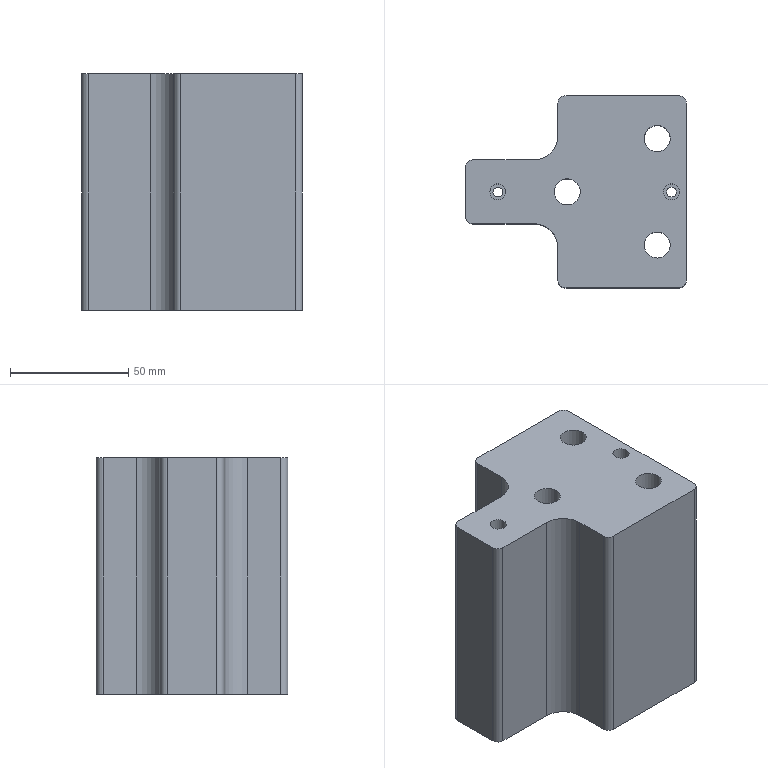Part | STEP file | lll_id3534_x_t | 1 solid | 41 faces | box 93.3 x 81 x 100 mm | volume 482036 mm3 | cylinder 22 | plane 17 | cone 2 | commonest cylinder face diameters 6 x6 11 x5 17 x3 4.1 x2 6.8 x2 8.506 x2
STEP:
#1=CARTESIAN_POINT('',(3880.992,0.002967,-7.5));
#2=VERTEX_POINT('',#1);
#3=CARTESIAN_POINT('',(3883.042,0.002967,-7.5));
#4=DIRECTION('',(0.000000008,0.,1.));
#5=DIRECTION('',(-1.,0.,0.000000008));
#6=AXIS2_PLACEMENT_3D('',#3,#4,#5);
#7=CIRCLE('',#6,2.05);
#8=EDGE_CURVE('',#2,#2,#7,.T.);
#9=ORIENTED_EDGE('',*,*,#8,.F.);
#10=EDGE_LOOP('',(#9));
#11=FACE_BOUND('',#10,.T.);
#12=CARTESIAN_POINT('',(3885.092,0.002967,29.5));
#13=VERTEX_POINT('',#12);
#14=CARTESIAN_POINT('',(3883.042,0.002967,29.5));
#15=DIRECTION('',(0.,0.,-1.));
#16=DIRECTION('',(1.,0.,0.));
#17=AXIS2_PLACEMENT_3D('',#14,#15,#16);
#18=CIRCLE('',#17,2.05);
#19=EDGE_CURVE('',#13,#13,#18,.T.);
#20=ORIENTED_EDGE('',*,*,#19,.F.);
#21=EDGE_LOOP('',(#20));
#22=FACE_BOUND('',#21,.T.);
#23=CARTESIAN_POINT('',(3883.042,0.002967,42.5));
#24=DIRECTION('',(0.,0.,-1.));
#25=DIRECTION('',(-1.,-0.0006834,0.));
#26=AXIS2_PLACEMENT_3D('',#23,#24,#25);
#27=CYLINDRICAL_SURFACE('',#26,2.05);
#28=ADVANCED_FACE('',(#11,#22),#27,.F.);
#29=CARTESIAN_POINT('',(3877.,17.,92.5));
#30=VERTEX_POINT('',#29);
#31=CARTESIAN_POINT('',(3877.,22.5,92.5));
#32=DIRECTION('',(0.,0.,1.));
#33=DIRECTION('',(0.,-1.,0.));
#34=AXIS2_PLACEMENT_3D('',#31,#32,#33);
#35=CIRCLE('',#34,5.5);
#36=EDGE_CURVE('',#30,#30,#35,.T.);
#37=ORIENTED_EDGE('',*,*,#36,.F.);
#38=EDGE_LOOP('',(#37));
#39=FACE_BOUND('',#38,.T.);
#40=CARTESIAN_POINT('',(3813.007,-0.001282,92.5));
#41=VERTEX_POINT('',#40);
#42=CARTESIAN_POINT('',(3809.607,-0.001282,92.5));
#43=DIRECTION('',(0.,0.,-1.));
#44=DIRECTION('',(1.,0.,0.));
#45=AXIS2_PLACEMENT_3D('',#42,#43,#44);
#46=CIRCLE('',#45,3.4);
#47=EDGE_CURVE('',#41,#41,#46,.T.);
#48=ORIENTED_EDGE('',*,*,#47,.T.);
#49=EDGE_LOOP('',(#48));
#50=FACE_BOUND('',#49,.T.);
#51=CARTESIAN_POINT('',(3879.642,0.0006437,92.5));
#52=VERTEX_POINT('',#51);
#53=CARTESIAN_POINT('',(3883.042,0.002967,92.5));
#54=DIRECTION('',(0.,0.,1.));
#55=DIRECTION('',(-1.,-0.0006834,0.));
#56=AXIS2_PLACEMENT_3D('',#53,#54,#55);
#57=CIRCLE('',#56,3.4);
#58=EDGE_CURVE('',#52,#52,#57,.T.);
#59=ORIENTED_EDGE('',*,*,#58,.F.);
#60=EDGE_LOOP('',(#59));
#61=FACE_BOUND('',#60,.T.);
#62=CARTESIAN_POINT('',(3796.,-10.5,92.5));
#63=VERTEX_POINT('',#62);
#64=CARTESIAN_POINT('',(3796.,10.5,92.5));
#65=VERTEX_POINT('',#64);
#66=CARTESIAN_POINT('',(3796.,236.7,92.5));
#67=DIRECTION('',(0.,1.,0.));
#68=VECTOR('',#67,1.);
#69=LINE('',#66,#68);
#70=EDGE_CURVE('',#63,#65,#69,.T.);
#71=ORIENTED_EDGE('',*,*,#70,.F.);
#72=CARTESIAN_POINT('',(3799.,-13.5,92.5));
#73=VERTEX_POINT('',#72);
#74=CARTESIAN_POINT('',(3799.,-10.5,92.5));
#75=DIRECTION('',(0.,0.,1.));
#76=DIRECTION('',(-1.,0.,0.));
#77=AXIS2_PLACEMENT_3D('',#74,#75,#76);
#78=CIRCLE('',#77,3.);
#79=EDGE_CURVE('',#63,#73,#78,.T.);
#80=ORIENTED_EDGE('',*,*,#79,.T.);
#81=CARTESIAN_POINT('',(3825.,-13.5,92.5));
#82=VERTEX_POINT('',#81);
#83=CARTESIAN_POINT('',(3587.234,-13.5,92.5));
#84=DIRECTION('',(-1.,0.,0.));
#85=VECTOR('',#84,1.);
#86=LINE('',#83,#85);
#87=EDGE_CURVE('',#82,#73,#86,.T.);
#88=ORIENTED_EDGE('',*,*,#87,.F.);
#89=CARTESIAN_POINT('',(3835.,-23.5,92.5));
#90=VERTEX_POINT('',#89);
#91=CARTESIAN_POINT('',(3825.,-23.5,92.5));
#92=DIRECTION('',(0.,0.,-1.));
#93=DIRECTION('',(-1.,0.,0.));
#94=AXIS2_PLACEMENT_3D('',#91,#92,#93);
#95=CIRCLE('',#94,10.);
#96=EDGE_CURVE('',#82,#90,#95,.T.);
#97=ORIENTED_EDGE('',*,*,#96,.T.);
#98=CARTESIAN_POINT('',(3835.,-37.5,92.5));
#99=VERTEX_POINT('',#98);
#100=CARTESIAN_POINT('',(3835.,236.7,92.5));
#101=DIRECTION('',(0.,1.,0.));
#102=VECTOR('',#101,1.);
#103=LINE('',#100,#102);
#104=EDGE_CURVE('',#99,#90,#103,.T.);
#105=ORIENTED_EDGE('',*,*,#104,.F.);
#106=CARTESIAN_POINT('',(3838.,-40.5,92.5));
#107=VERTEX_POINT('',#106);
#108=CARTESIAN_POINT('',(3838.,-37.5,92.5));
#109=DIRECTION('',(0.,0.,1.));
#110=DIRECTION('',(-1.,0.,0.));
#111=AXIS2_PLACEMENT_3D('',#108,#109,#110);
#112=CIRCLE('',#111,3.);
#113=EDGE_CURVE('',#99,#107,#112,.T.);
#114=ORIENTED_EDGE('',*,*,#113,.T.);
#115=CARTESIAN_POINT('',(3886.3,-40.5,92.5));
#116=VERTEX_POINT('',#115);
#117=CARTESIAN_POINT('',(14362.883,-40.5,92.5));
#118=DIRECTION('',(1.,0.,0.));
#119=VECTOR('',#118,1.);
#120=LINE('',#117,#119);
#121=EDGE_CURVE('',#107,#116,#120,.T.);
#122=ORIENTED_EDGE('',*,*,#121,.T.);
#123=CARTESIAN_POINT('',(3889.3,-37.5,92.5));
#124=VERTEX_POINT('',#123);
#125=CARTESIAN_POINT('',(3886.3,-37.5,92.5));
#126=DIRECTION('',(0.,0.,1.));
#127=DIRECTION('',(-1.,0.,0.));
#128=AXIS2_PLACEMENT_3D('',#125,#126,#127);
#129=CIRCLE('',#128,3.);
#130=EDGE_CURVE('',#116,#124,#129,.T.);
#131=ORIENTED_EDGE('',*,*,#130,.T.);
#132=CARTESIAN_POINT('',(3889.3,37.5,92.5));
#133=VERTEX_POINT('',#132);
#134=CARTESIAN_POINT('',(3889.3,-17.5,92.5));
#135=DIRECTION('',(0.,-1.,0.));
#136=VECTOR('',#135,1.);
#137=LINE('',#134,#136);
#138=EDGE_CURVE('',#133,#124,#137,.T.);
#139=ORIENTED_EDGE('',*,*,#138,.F.);
#140=CARTESIAN_POINT('',(3886.3,40.5,92.5));
#141=VERTEX_POINT('',#140);
#142=CARTESIAN_POINT('',(3886.3,37.5,92.5));
#143=DIRECTION('',(0.,0.,1.));
#144=DIRECTION('',(-1.,0.,0.));
#145=AXIS2_PLACEMENT_3D('',#142,#143,#144);
#146=CIRCLE('',#145,3.);
#147=EDGE_CURVE('',#133,#141,#146,.T.);
#148=ORIENTED_EDGE('',*,*,#147,.T.);
#149=CARTESIAN_POINT('',(3838.,40.5,92.5));
#150=VERTEX_POINT('',#149);
#151=CARTESIAN_POINT('',(3587.234,40.5,92.5));
#152=DIRECTION('',(1.,0.,0.));
#153=VECTOR('',#152,1.);
#154=LINE('',#151,#153);
#155=EDGE_CURVE('',#150,#141,#154,.T.);
#156=ORIENTED_EDGE('',*,*,#155,.F.);
#157=CARTESIAN_POINT('',(3835.,37.5,92.5));
#158=VERTEX_POINT('',#157);
#159=CARTESIAN_POINT('',(3838.,37.5,92.5));
#160=DIRECTION('',(0.,0.,1.));
#161=DIRECTION('',(-1.,0.,0.));
#162=AXIS2_PLACEMENT_3D('',#159,#160,#161);
#163=CIRCLE('',#162,3.);
#164=EDGE_CURVE('',#150,#158,#163,.T.);
#165=ORIENTED_EDGE('',*,*,#164,.T.);
#166=CARTESIAN_POINT('',(3835.,23.5,92.5));
#167=VERTEX_POINT('',#166);
#168=CARTESIAN_POINT('',(3835.,38.,92.5));
#169=DIRECTION('',(0.,-1.,0.));
#170=VECTOR('',#169,1.);
#171=LINE('',#168,#170);
#172=EDGE_CURVE('',#158,#167,#171,.T.);
#173=ORIENTED_EDGE('',*,*,#172,.T.);
#174=CARTESIAN_POINT('',(3825.,13.5,92.5));
#175=VERTEX_POINT('',#174);
#176=CARTESIAN_POINT('',(3825.,23.5,92.5));
#177=DIRECTION('',(0.,0.,-1.));
#178=DIRECTION('',(-1.,0.,0.));
#179=AXIS2_PLACEMENT_3D('',#176,#177,#178);
#180=CIRCLE('',#179,10.);
#181=EDGE_CURVE('',#167,#175,#180,.T.);
#182=ORIENTED_EDGE('',*,*,#181,.T.);
#183=CARTESIAN_POINT('',(3799.,13.5,92.5));
#184=VERTEX_POINT('',#183);
#185=CARTESIAN_POINT('',(3831.,13.5,92.5));
#186=DIRECTION('',(-1.,0.,0.));
#187=VECTOR('',#186,1.);
#188=LINE('',#185,#187);
#189=EDGE_CURVE('',#175,#184,#188,.T.);
#190=ORIENTED_EDGE('',*,*,#189,.T.);
#191=CARTESIAN_POINT('',(3799.,10.5,92.5));
#192=DIRECTION('',(0.,0.,1.));
#193=DIRECTION('',(-1.,0.,0.));
#194=AXIS2_PLACEMENT_3D('',#191,#192,#193);
#195=CIRCLE('',#194,3.);
#196=EDGE_CURVE('',#184,#65,#195,.T.);
#197=ORIENTED_EDGE('',*,*,#196,.T.);
#198=EDGE_LOOP('',(#71,#80,#88,#97,#105,#114,#122,#131,#139,#148,#156,#165,#173,#182,#190,#197));
#199=FACE_BOUND('',#198,.T.);
#200=CARTESIAN_POINT('',(3876.982,-28.02,92.5));
#201=VERTEX_POINT('',#200);
#202=CARTESIAN_POINT('',(3876.982,-22.52,92.5));
#203=DIRECTION('',(0.,0.,-1.));
#204=DIRECTION('',(0.,-1.,0.));
#205=AXIS2_PLACEMENT_3D('',#202,#203,#204);
#206=CIRCLE('',#205,5.5);
#207=EDGE_CURVE('',#201,#201,#206,.T.);
#208=ORIENTED_EDGE('',*,*,#207,.T.);
#209=EDGE_LOOP('',(#208));
#210=FACE_BOUND('',#209,.T.);
#211=CARTESIAN_POINT('',(3833.482,-0.01982,92.5));
#212=VERTEX_POINT('',#211);
#213=CARTESIAN_POINT('',(3838.982,-0.01982,92.5));
#214=DIRECTION('',(0.,0.,1.));
#215=DIRECTION('',(-1.,0.,0.));
#216=AXIS2_PLACEMENT_3D('',#213,#214,#215);
#217=CIRCLE('',#216,5.5);
#218=EDGE_CURVE('',#212,#212,#217,.T.);
#219=ORIENTED_EDGE('',*,*,#218,.F.);
#220=EDGE_LOOP('',(#219));
#221=FACE_BOUND('',#220,.T.);
#222=CARTESIAN_POINT('',(3587.234,236.7,92.5));
#223=DIRECTION('',(0.,0.,1.));
#224=DIRECTION('',(0.,-1.,0.));
#225=AXIS2_PLACEMENT_3D('',#222,#223,#224);
#226=PLANE('',#225);
#227=ADVANCED_FACE('',(#39,#50,#61,#199,#210,#221),#226,.T.);
#228=CARTESIAN_POINT('',(3838.982,8.48,-7.5));
#229=VERTEX_POINT('',#228);
#230=CARTESIAN_POINT('',(3838.982,-0.01982,-7.5));
#231=DIRECTION('',(0.,0.000000008,-1.));
#232=DIRECTION('',(0.,1.,0.000000008));
#233=AXIS2_PLACEMENT_3D('',#230,#231,#232);
#234=CIRCLE('',#233,8.5);
#235=EDGE_CURVE('',#229,#229,#234,.T.);
#236=ORIENTED_EDGE('',*,*,#235,.F.);
#237=EDGE_LOOP('',(#236));
#238=FACE_BOUND('',#237,.T.);
#239=CARTESIAN_POINT('',(3814.542,0.002967,-7.5));
#240=VERTEX_POINT('',#239);
#241=CARTESIAN_POINT('',(3820.042,0.002967,-7.5));
#242=DIRECTION('',(0.000000008,0.,1.));
#243=DIRECTION('',(-1.,0.,0.000000008));
#244=AXIS2_PLACEMENT_3D('',#241,#242,#243);
#245=CIRCLE('',#244,5.5);
#246=EDGE_CURVE('',#240,#240,#245,.T.);
#247=ORIENTED_EDGE('',*,*,#246,.T.);
#248=EDGE_LOOP('',(#247));
#249=FACE_BOUND('',#248,.T.);
#250=CARTESIAN_POINT('',(3862.542,0.002967,-7.5));
#251=VERTEX_POINT('',#250);
#252=CARTESIAN_POINT('',(3868.042,0.002967,-7.5));
#253=DIRECTION('',(0.000000008,0.,1.));
#254=DIRECTION('',(-1.,0.,0.000000008));
#255=AXIS2_PLACEMENT_3D('',#252,#253,#254);
#256=CIRCLE('',#255,5.5);
#257=EDGE_CURVE('',#251,#251,#256,.T.);
#258=ORIENTED_EDGE('',*,*,#257,.T.);
#259=EDGE_LOOP('',(#258));
#260=FACE_BOUND('',#259,.T.);
#261=CARTESIAN_POINT('',(3868.482,-22.52,-7.5));
#262=VERTEX_POINT('',#261);
#263=CARTESIAN_POINT('',(3876.982,-22.52,-7.5));
#264=DIRECTION('',(0.000000008,0.,1.));
#265=DIRECTION('',(-1.,0.,0.000000008));
#266=AXIS2_PLACEMENT_3D('',#263,#264,#265);
#267=CIRCLE('',#266,8.5);
#268=EDGE_CURVE('',#262,#262,#267,.T.);
#269=ORIENTED_EDGE('',*,*,#268,.T.);
#270=EDGE_LOOP('',(#269));
#271=FACE_BOUND('',#270,.T.);
#272=ORIENTED_EDGE('',*,*,#8,.T.);
#273=EDGE_LOOP('',(#272));
#274=FACE_BOUND('',#273,.T.);
#275=CARTESIAN_POINT('',(3868.5,22.5,-7.5));
#276=VERTEX_POINT('',#275);
#277=CARTESIAN_POINT('',(3877.,22.5,-7.5));
#278=DIRECTION('',(0.000000008,0.,1.));
#279=DIRECTION('',(-1.,0.,0.000000008));
#280=AXIS2_PLACEMENT_3D('',#277,#278,#279);
#281=CIRCLE('',#280,8.5);
#282=EDGE_CURVE('',#276,#276,#281,.T.);
#283=ORIENTED_EDGE('',*,*,#282,.T.);
#284=EDGE_LOOP('',(#283));
#285=FACE_BOUND('',#284,.T.);
#286=CARTESIAN_POINT('',(3807.557,-0.001282,-7.5));
#287=VERTEX_POINT('',#286);
#288=CARTESIAN_POINT('',(3809.607,-0.001282,-7.5));
#289=DIRECTION('',(0.000000008,0.,1.));
#290=DIRECTION('',(-1.,0.,0.000000008));
#291=AXIS2_PLACEMENT_3D('',#288,#289,#290);
#292=CIRCLE('',#291,2.05);
#293=EDGE_CURVE('',#287,#287,#292,.T.);
#294=ORIENTED_EDGE('',*,*,#293,.T.);
#295=EDGE_LOOP('',(#294));
#296=FACE_BOUND('',#295,.T.);
#297=CARTESIAN_POINT('',(3825.,-13.5,-7.5));
#298=VERTEX_POINT('',#297);
#299=CARTESIAN_POINT('',(3799.,-13.5,-7.5));
#300=VERTEX_POINT('',#299);
#301=CARTESIAN_POINT('',(3633.202,-13.5,-7.5));
#302=DIRECTION('',(-1.,0.,0.));
#303=VECTOR('',#302,1.);
#304=LINE('',#301,#303);
#305=EDGE_CURVE('',#298,#300,#304,.T.);
#306=ORIENTED_EDGE('',*,*,#305,.T.);
#307=CARTESIAN_POINT('',(3796.,-10.5,-7.5));
#308=VERTEX_POINT('',#307);
#309=CARTESIAN_POINT('',(3799.,-10.5,-7.5));
#310=DIRECTION('',(0.,0.000000008,-1.));
#311=DIRECTION('',(0.,1.,0.000000008));
#312=AXIS2_PLACEMENT_3D('',#309,#310,#311);
#313=CIRCLE('',#312,3.);
#314=EDGE_CURVE('',#300,#308,#313,.T.);
#315=ORIENTED_EDGE('',*,*,#314,.T.);
#316=CARTESIAN_POINT('',(3796.,10.5,-7.5));
#317=VERTEX_POINT('',#316);
#318=CARTESIAN_POINT('',(3796.,65.944,-7.5));
#319=DIRECTION('',(0.,1.,0.000000008));
#320=VECTOR('',#319,1.);
#321=LINE('',#318,#320);
#322=EDGE_CURVE('',#308,#317,#321,.T.);
#323=ORIENTED_EDGE('',*,*,#322,.T.);
#324=CARTESIAN_POINT('',(3799.,13.5,-7.5));
#325=VERTEX_POINT('',#324);
#326=CARTESIAN_POINT('',(3799.,10.5,-7.5));
#327=DIRECTION('',(0.,0.000000008,-1.));
#328=DIRECTION('',(0.,1.,0.000000008));
#329=AXIS2_PLACEMENT_3D('',#326,#327,#328);
#330=CIRCLE('',#329,3.);
#331=EDGE_CURVE('',#317,#325,#330,.T.);
#332=ORIENTED_EDGE('',*,*,#331,.T.);
#333=CARTESIAN_POINT('',(3825.,13.5,-7.5));
#334=VERTEX_POINT('',#333);
#335=CARTESIAN_POINT('',(3831.,13.5,-7.5));
#336=DIRECTION('',(-1.,0.,0.));
#337=VECTOR('',#336,1.);
#338=LINE('',#335,#337);
#339=EDGE_CURVE('',#334,#325,#338,.T.);
#340=ORIENTED_EDGE('',*,*,#339,.F.);
#341=CARTESIAN_POINT('',(3835.,23.5,-7.5));
#342=VERTEX_POINT('',#341);
#343=CARTESIAN_POINT('',(3825.,23.5,-7.5));
#344=DIRECTION('',(0.,-0.000000008,1.));
#345=DIRECTION('',(0.,1.,0.000000008));
#346=AXIS2_PLACEMENT_3D('',#343,#344,#345);
#347=CIRCLE('',#346,10.);
#348=EDGE_CURVE('',#334,#342,#347,.T.);
#349=ORIENTED_EDGE('',*,*,#348,.T.);
#350=CARTESIAN_POINT('',(3835.,37.5,-7.5));
#351=VERTEX_POINT('',#350);
#352=CARTESIAN_POINT('',(3835.,38.,-7.5));
#353=DIRECTION('',(0.,-1.,-0.000000008));
#354=VECTOR('',#353,1.);
#355=LINE('',#352,#354);
#356=EDGE_CURVE('',#351,#342,#355,.T.);
#357=ORIENTED_EDGE('',*,*,#356,.F.);
#358=CARTESIAN_POINT('',(3838.,40.5,-7.5));
#359=VERTEX_POINT('',#358);
#360=CARTESIAN_POINT('',(3838.,37.5,-7.5));
#361=DIRECTION('',(0.,0.000000008,-1.));
#362=DIRECTION('',(0.,1.,0.000000008));
#363=AXIS2_PLACEMENT_3D('',#360,#361,#362);
#364=CIRCLE('',#363,3.);
#365=EDGE_CURVE('',#351,#359,#364,.T.);
#366=ORIENTED_EDGE('',*,*,#365,.T.);
#367=CARTESIAN_POINT('',(3886.3,40.5,-7.5));
#368=VERTEX_POINT('',#367);
#369=CARTESIAN_POINT('',(3633.202,40.5,-7.5));
#370=DIRECTION('',(1.,0.,0.));
#371=VECTOR('',#370,1.);
#372=LINE('',#369,#371);
#373=EDGE_CURVE('',#359,#368,#372,.T.);
#374=ORIENTED_EDGE('',*,*,#373,.T.);
#375=CARTESIAN_POINT('',(3889.3,37.5,-7.5));
#376=VERTEX_POINT('',#375);
#377=CARTESIAN_POINT('',(3886.3,37.5,-7.5));
#378=DIRECTION('',(0.,0.000000008,-1.));
#379=DIRECTION('',(0.,1.,0.000000008));
#380=AXIS2_PLACEMENT_3D('',#377,#378,#379);
#381=CIRCLE('',#380,3.);
#382=EDGE_CURVE('',#368,#376,#381,.T.);
#383=ORIENTED_EDGE('',*,*,#382,.T.);
#384=CARTESIAN_POINT('',(3889.3,-37.5,-7.5));
#385=VERTEX_POINT('',#384);
#386=CARTESIAN_POINT('',(3889.3,-17.5,-7.5));
#387=DIRECTION('',(0.,-1.,-0.000000008));
#388=VECTOR('',#387,1.);
#389=LINE('',#386,#388);
#390=EDGE_CURVE('',#376,#385,#389,.T.);
#391=ORIENTED_EDGE('',*,*,#390,.T.);
#392=CARTESIAN_POINT('',(3886.3,-40.5,-7.5));
#393=VERTEX_POINT('',#392);
#394=CARTESIAN_POINT('',(3886.3,-37.5,-7.5));
#395=DIRECTION('',(0.,0.000000008,-1.));
#396=DIRECTION('',(0.,1.,0.000000008));
#397=AXIS2_PLACEMENT_3D('',#394,#395,#396);
#398=CIRCLE('',#397,3.);
#399=EDGE_CURVE('',#385,#393,#398,.T.);
#400=ORIENTED_EDGE('',*,*,#399,.T.);
#401=CARTESIAN_POINT('',(3838.,-40.5,-7.5));
#402=VERTEX_POINT('',#401);
#403=CARTESIAN_POINT('',(14362.883,-40.5,-7.5));
#404=DIRECTION('',(1.,0.,0.));
#405=VECTOR('',#404,1.);
#406=LINE('',#403,#405);
#407=EDGE_CURVE('',#402,#393,#406,.T.);
#408=ORIENTED_EDGE('',*,*,#407,.F.);
#409=CARTESIAN_POINT('',(3835.,-37.5,-7.5));
#410=VERTEX_POINT('',#409);
#411=CARTESIAN_POINT('',(3838.,-37.5,-7.5));
#412=DIRECTION('',(0.,0.000000008,-1.));
#413=DIRECTION('',(0.,1.,0.000000008));
#414=AXIS2_PLACEMENT_3D('',#411,#412,#413);
#415=CIRCLE('',#414,3.);
#416=EDGE_CURVE('',#402,#410,#415,.T.);
#417=ORIENTED_EDGE('',*,*,#416,.T.);
#418=CARTESIAN_POINT('',(3835.,-23.5,-7.5));
#419=VERTEX_POINT('',#418);
#420=CARTESIAN_POINT('',(3835.,65.944,-7.5));
#421=DIRECTION('',(0.,1.,0.000000008));
#422=VECTOR('',#421,1.);
#423=LINE('',#420,#422);
#424=EDGE_CURVE('',#410,#419,#423,.T.);
#425=ORIENTED_EDGE('',*,*,#424,.T.);
#426=CARTESIAN_POINT('',(3825.,-23.5,-7.5));
#427=DIRECTION('',(0.,-0.000000008,1.));
#428=DIRECTION('',(0.,1.,0.000000008));
#429=AXIS2_PLACEMENT_3D('',#426,#427,#428);
#430=CIRCLE('',#429,10.);
#431=EDGE_CURVE('',#419,#298,#430,.T.);
#432=ORIENTED_EDGE('',*,*,#431,.T.);
#433=EDGE_LOOP('',(#306,#315,#323,#332,#340,#349,#357,#366,#374,#383,#391,#400,#408,#417,#425,#432));
#434=FACE_BOUND('',#433,.T.);
#435=CARTESIAN_POINT('',(3633.202,65.944,-7.5));
#436=DIRECTION('',(0.,-0.000000008,1.));
#437=DIRECTION('',(0.,1.,0.000000008));
#438=AXIS2_PLACEMENT_3D('',#435,#436,#437);
#439=PLANE('',#438);
#440=ADVANCED_FACE('',(#238,#249,#260,#271,#274,#285,#296,#434),#439,.F.);
#441=ORIENTED_EDGE('',*,*,#87,.T.);
#442=CARTESIAN_POINT('',(3799.,-13.5,2.5));
#443=DIRECTION('',(0.,0.,-1.));
#444=VECTOR('',#443,1.);
#445=LINE('',#442,#444);
#446=EDGE_CURVE('',#73,#300,#445,.T.);
#447=ORIENTED_EDGE('',*,*,#446,.T.);
#448=ORIENTED_EDGE('',*,*,#305,.F.);
#449=CARTESIAN_POINT('',(3825.,-13.5,2.5));
#450=DIRECTION('',(0.,0.,1.));
#451=VECTOR('',#450,1.);
#452=LINE('',#449,#451);
#453=EDGE_CURVE('',#298,#82,#452,.T.);
#454=ORIENTED_EDGE('',*,*,#453,.T.);
#455=EDGE_LOOP('',(#441,#447,#448,#454));
#456=FACE_OUTER_BOUND('',#455,.T.);
#457=CARTESIAN_POINT('',(3831.,-13.5,2.5));
#458=DIRECTION('',(0.,-1.,0.));
#459=DIRECTION('',(-1.,0.,0.));
#460=AXIS2_PLACEMENT_3D('',#457,#458,#459);
#461=PLANE('',#460);
#462=ADVANCED_FACE('',(#456),#461,.T.);
#463=ORIENTED_EDGE('',*,*,#104,.T.);
#464=CARTESIAN_POINT('',(3835.,-23.5,2.5));
#465=DIRECTION('',(0.,0.,-1.));
#466=VECTOR('',#465,1.);
#467=LINE('',#464,#466);
#468=EDGE_CURVE('',#90,#419,#467,.T.);
#469=ORIENTED_EDGE('',*,*,#468,.T.);
#470=ORIENTED_EDGE('',*,*,#424,.F.);
#471=CARTESIAN_POINT('',(3835.,-37.5,2.5));
#472=DIRECTION('',(0.,0.,1.));
#473=VECTOR('',#472,1.);
#474=LINE('',#471,#473);
#475=EDGE_CURVE('',#410,#99,#474,.T.);
#476=ORIENTED_EDGE('',*,*,#475,.T.);
#477=EDGE_LOOP('',(#463,#469,#470,#476));
#478=FACE_OUTER_BOUND('',#477,.T.);
#479=CARTESIAN_POINT('',(3835.,-38.,2.5));
#480=DIRECTION('',(-1.,0.,0.));
#481=DIRECTION('',(0.,1.,0.));
#482=AXIS2_PLACEMENT_3D('',#479,#480,#481);
#483=PLANE('',#482);
#484=ADVANCED_FACE('',(#478),#483,.T.);
#485=ORIENTED_EDGE('',*,*,#121,.F.);
#486=CARTESIAN_POINT('',(3838.,-40.5,2.5));
#487=DIRECTION('',(0.,0.,-1.));
#488=VECTOR('',#487,1.);
#489=LINE('',#486,#488);
#490=EDGE_CURVE('',#107,#402,#489,.T.);
#491=ORIENTED_EDGE('',*,*,#490,.T.);
#492=ORIENTED_EDGE('',*,*,#407,.T.);
#493=CARTESIAN_POINT('',(3886.3,-40.5,2.5));
#494=DIRECTION('',(0.,0.,1.));
#495=VECTOR('',#494,1.);
#496=LINE('',#493,#495);
#497=EDGE_CURVE('',#393,#116,#496,.T.);
#498=ORIENTED_EDGE('',*,*,#497,.T.);
#499=EDGE_LOOP('',(#485,#491,#492,#498));
#500=FACE_OUTER_BOUND('',#499,.T.);
#501=CARTESIAN_POINT('',(14362.883,-40.5,2.5));
#502=DIRECTION('',(0.,1.,0.));
#503=DIRECTION('',(1.,0.,0.));
#504=AXIS2_PLACEMENT_3D('',#501,#502,#503);
#505=PLANE('',#504);
#506=ADVANCED_FACE('',(#500),#505,.F.);
#507=ORIENTED_EDGE('',*,*,#138,.T.);
#508=CARTESIAN_POINT('',(3889.3,-37.5,2.5));
#509=DIRECTION('',(0.,0.,-1.));
#510=VECTOR('',#509,1.);
#511=LINE('',#508,#510);
#512=EDGE_CURVE('',#124,#385,#511,.T.);
#513=ORIENTED_EDGE('',*,*,#512,.T.);
#514=ORIENTED_EDGE('',*,*,#390,.F.);
#515=CARTESIAN_POINT('',(3889.3,37.5,2.5));
#516=DIRECTION('',(0.,0.,1.));
#517=VECTOR('',#516,1.);
#518=LINE('',#515,#517);
#519=EDGE_CURVE('',#376,#133,#518,.T.);
#520=ORIENTED_EDGE('',*,*,#519,.T.);
#521=EDGE_LOOP('',(#507,#513,#514,#520));
#522=FACE_OUTER_BOUND('',#521,.T.);
#523=CARTESIAN_POINT('',(3889.3,-17.5,2.5));
#524=DIRECTION('',(1.,0.,0.));
#525=DIRECTION('',(0.,-1.,0.));
#526=AXIS2_PLACEMENT_3D('',#523,#524,#525);
#527=PLANE('',#526);
#528=ADVANCED_FACE('',(#522),#527,.T.);
#529=ORIENTED_EDGE('',*,*,#373,.F.);
#530=CARTESIAN_POINT('',(3838.,40.5,2.5));
#531=DIRECTION('',(0.,0.,1.));
#532=VECTOR('',#531,1.);
#533=LINE('',#530,#532);
#534=EDGE_CURVE('',#359,#150,#533,.T.);
#535=ORIENTED_EDGE('',*,*,#534,.T.);
#536=ORIENTED_EDGE('',*,*,#155,.T.);
#537=CARTESIAN_POINT('',(3886.3,40.5,2.5));
#538=DIRECTION('',(0.,0.,-1.));
#539=VECTOR('',#538,1.);
#540=LINE('',#537,#539);
#541=EDGE_CURVE('',#141,#368,#540,.T.);
#542=ORIENTED_EDGE('',*,*,#541,.T.);
#543=EDGE_LOOP('',(#529,#535,#536,#542));
#544=FACE_OUTER_BOUND('',#543,.T.);
#545=CARTESIAN_POINT('',(14362.883,40.5,2.5));
#546=DIRECTION('',(0.,1.,0.));
#547=DIRECTION('',(1.,0.,0.));
#548=AXIS2_PLACEMENT_3D('',#545,#546,#547);
#549=PLANE('',#548);
#550=ADVANCED_FACE('',(#544),#549,.T.);
#551=ORIENTED_EDGE('',*,*,#356,.T.);
#552=CARTESIAN_POINT('',(3835.,23.5,2.5));
#553=DIRECTION('',(0.,0.,1.));
#554=VECTOR('',#553,1.);
#555=LINE('',#552,#554);
#556=EDGE_CURVE('',#342,#167,#555,.T.);
#557=ORIENTED_EDGE('',*,*,#556,.T.);
#558=ORIENTED_EDGE('',*,*,#172,.F.);
#559=CARTESIAN_POINT('',(3835.,37.5,2.5));
#560=DIRECTION('',(0.,0.,-1.));
#561=VECTOR('',#560,1.);
#562=LINE('',#559,#561);
#563=EDGE_CURVE('',#158,#351,#562,.T.);
#564=ORIENTED_EDGE('',*,*,#563,.T.);
#565=EDGE_LOOP('',(#551,#557,#558,#564));
#566=FACE_OUTER_BOUND('',#565,.T.);
#567=CARTESIAN_POINT('',(3835.,38.,2.5));
#568=DIRECTION('',(1.,0.,0.));
#569=DIRECTION('',(0.,-1.,0.));
#570=AXIS2_PLACEMENT_3D('',#567,#568,#569);
#571=PLANE('',#570);
#572=ADVANCED_FACE('',(#566),#571,.F.);
#573=ORIENTED_EDGE('',*,*,#339,.T.);
#574=CARTESIAN_POINT('',(3799.,13.5,2.5));
#575=DIRECTION('',(0.,0.,1.));
#576=VECTOR('',#575,1.);
#577=LINE('',#574,#576);
#578=EDGE_CURVE('',#325,#184,#577,.T.);
#579=ORIENTED_EDGE('',*,*,#578,.T.);
#580=ORIENTED_EDGE('',*,*,#189,.F.);
#581=CARTESIAN_POINT('',(3825.,13.5,2.5));
#582=DIRECTION('',(0.,0.,-1.));
#583=VECTOR('',#582,1.);
#584=LINE('',#581,#583);
#585=EDGE_CURVE('',#175,#334,#584,.T.);
#586=ORIENTED_EDGE('',*,*,#585,.T.);
#587=EDGE_LOOP('',(#573,#579,#580,#586));
#588=FACE_OUTER_BOUND('',#587,.T.);
#589=CARTESIAN_POINT('',(3831.,13.5,2.5));
#590=DIRECTION('',(0.,-1.,0.));
#591=DIRECTION('',(-1.,0.,0.));
#592=AXIS2_PLACEMENT_3D('',#589,#590,#591);
#593=PLANE('',#592);
#594=ADVANCED_FACE('',(#588),#593,.F.);
#595=ORIENTED_EDGE('',*,*,#322,.F.);
#596=CARTESIAN_POINT('',(3796.,-10.5,2.5));
#597=DIRECTION('',(0.,0.,1.));
#598=VECTOR('',#597,1.);
#599=LINE('',#596,#598);
#600=EDGE_CURVE('',#308,#63,#599,.T.);
#601=ORIENTED_EDGE('',*,*,#600,.T.);
#602=ORIENTED_EDGE('',*,*,#70,.T.);
#603=CARTESIAN_POINT('',(3796.,10.5,2.5));
#604=DIRECTION('',(0.,0.,-1.));
#605=VECTOR('',#604,1.);
#606=LINE('',#603,#605);
#607=EDGE_CURVE('',#65,#317,#606,.T.);
#608=ORIENTED_EDGE('',*,*,#607,.T.);
#609=EDGE_LOOP('',(#595,#601,#602,#608));
#610=FACE_OUTER_BOUND('',#609,.T.);
#611=CARTESIAN_POINT('',(3796.,-13712.786,2.5));
#612=DIRECTION('',(-1.,0.,0.));
#613=DIRECTION('',(0.,1.,0.));
#614=AXIS2_PLACEMENT_3D('',#611,#612,#613);
#615=PLANE('',#614);
#616=ADVANCED_FACE('',(#610),#615,.T.);
#617=ORIENTED_EDGE('',*,*,#399,.F.);
#618=ORIENTED_EDGE('',*,*,#512,.F.);
#619=ORIENTED_EDGE('',*,*,#130,.F.);
#620=ORIENTED_EDGE('',*,*,#497,.F.);
#621=EDGE_LOOP('',(#617,#618,#619,#620));
#622=FACE_OUTER_BOUND('',#621,.T.);
#623=CARTESIAN_POINT('',(3886.3,-37.5,2.5));
#624=DIRECTION('',(0.,0.,-1.));
#625=DIRECTION('',(1.,0.,0.));
#626=AXIS2_PLACEMENT_3D('',#623,#624,#625);
#627=CYLINDRICAL_SURFACE('',#626,3.);
#628=ADVANCED_FACE('',(#622),#627,.T.);
#629=ORIENTED_EDGE('',*,*,#147,.F.);
#630=ORIENTED_EDGE('',*,*,#519,.F.);
#631=ORIENTED_EDGE('',*,*,#382,.F.);
#632=ORIENTED_EDGE('',*,*,#541,.F.);
#633=EDGE_LOOP('',(#629,#630,#631,#632));
#634=FACE_OUTER_BOUND('',#633,.T.);
#635=CARTESIAN_POINT('',(3886.3,37.5,2.5));
#636=DIRECTION('',(0.,0.,-1.));
#637=DIRECTION('',(1.,0.,0.));
#638=AXIS2_PLACEMENT_3D('',#635,#636,#637);
#639=CYLINDRICAL_SURFACE('',#638,3.);
#640=ADVANCED_FACE('',(#634),#639,.T.);
#641=ORIENTED_EDGE('',*,*,#365,.F.);
#642=ORIENTED_EDGE('',*,*,#563,.F.);
#643=ORIENTED_EDGE('',*,*,#164,.F.);
#644=ORIENTED_EDGE('',*,*,#534,.F.);
#645=EDGE_LOOP('',(#641,#642,#643,#644));
#646=FACE_OUTER_BOUND('',#645,.T.);
#647=CARTESIAN_POINT('',(3838.,37.5,2.5));
#648=DIRECTION('',(0.,0.,-1.));
#649=DIRECTION('',(1.,0.,0.));
#650=AXIS2_PLACEMENT_3D('',#647,#648,#649);
#651=CYLINDRICAL_SURFACE('',#650,3.);
#652=ADVANCED_FACE('',(#646),#651,.T.);
#653=ORIENTED_EDGE('',*,*,#113,.F.);
#654=ORIENTED_EDGE('',*,*,#475,.F.);
#655=ORIENTED_EDGE('',*,*,#416,.F.);
#656=ORIENTED_EDGE('',*,*,#490,.F.);
#657=EDGE_LOOP('',(#653,#654,#655,#656));
#658=FACE_OUTER_BOUND('',#657,.T.);
#659=CARTESIAN_POINT('',(3838.,-37.5,2.5));
#660=DIRECTION('',(0.,0.,1.));
#661=DIRECTION('',(-1.,0.,0.));
#662=AXIS2_PLACEMENT_3D('',#659,#660,#661);
#663=CYLINDRICAL_SURFACE('',#662,3.);
#664=ADVANCED_FACE('',(#658),#663,.T.);
#665=ORIENTED_EDGE('',*,*,#431,.F.);
#666=ORIENTED_EDGE('',*,*,#468,.F.);
#667=ORIENTED_EDGE('',*,*,#96,.F.);
#668=ORIENTED_EDGE('',*,*,#453,.F.);
#669=EDGE_LOOP('',(#665,#666,#667,#668));
#670=FACE_OUTER_BOUND('',#669,.T.);
#671=CARTESIAN_POINT('',(3825.,-23.5,2.5));
#672=DIRECTION('',(0.,0.,1.));
#673=DIRECTION('',(-1.,0.,0.));
#674=AXIS2_PLACEMENT_3D('',#671,#672,#673);
#675=CYLINDRICAL_SURFACE('',#674,10.);
#676=ADVANCED_FACE('',(#670),#675,.F.);
#677=ORIENTED_EDGE('',*,*,#348,.F.);
#678=ORIENTED_EDGE('',*,*,#585,.F.);
#679=ORIENTED_EDGE('',*,*,#181,.F.);
#680=ORIENTED_EDGE('',*,*,#556,.F.);
#681=EDGE_LOOP('',(#677,#678,#679,#680));
#682=FACE_OUTER_BOUND('',#681,.T.);
#683=CARTESIAN_POINT('',(3825.,23.5,2.5));
#684=DIRECTION('',(0.,0.,1.));
#685=DIRECTION('',(-1.,0.,0.));
#686=AXIS2_PLACEMENT_3D('',#683,#684,#685);
#687=CYLINDRICAL_SURFACE('',#686,10.);
#688=ADVANCED_FACE('',(#682),#687,.F.);
#689=ORIENTED_EDGE('',*,*,#58,.T.);
#690=EDGE_LOOP('',(#689));
#691=FACE_BOUND('',#690,.T.);
#692=CARTESIAN_POINT('',(3886.442,0.005291,29.5));
#693=VERTEX_POINT('',#692);
#694=CARTESIAN_POINT('',(3883.042,0.002967,29.5));
#695=DIRECTION('',(0.,0.,1.));
#696=DIRECTION('',(1.,0.0006834,0.));
#697=AXIS2_PLACEMENT_3D('',#694,#695,#696);
#698=CIRCLE('',#697,3.4);
#699=EDGE_CURVE('',#693,#693,#698,.T.);
#700=ORIENTED_EDGE('',*,*,#699,.F.);
#701=EDGE_LOOP('',(#700));
#702=FACE_BOUND('',#701,.T.);
#703=CARTESIAN_POINT('',(3883.042,0.002967,42.5));
#704=DIRECTION('',(0.,0.,1.));
#705=DIRECTION('',(1.,0.0006834,0.));
#706=AXIS2_PLACEMENT_3D('',#703,#704,#705);
#707=CYLINDRICAL_SURFACE('',#706,3.4);
#708=ADVANCED_FACE('',(#691,#702),#707,.F.);
#709=CARTESIAN_POINT('',(3807.557,-0.001282,29.5));
#710=VERTEX_POINT('',#709);
#711=CARTESIAN_POINT('',(3809.607,-0.001282,29.5));
#712=DIRECTION('',(0.,0.,1.));
#713=DIRECTION('',(-1.,0.,0.));
#714=AXIS2_PLACEMENT_3D('',#711,#712,#713);
#715=CIRCLE('',#714,2.05);
#716=EDGE_CURVE('',#710,#710,#715,.T.);
#717=ORIENTED_EDGE('',*,*,#716,.T.);
#718=EDGE_LOOP('',(#717));
#719=FACE_BOUND('',#718,.T.);
#720=ORIENTED_EDGE('',*,*,#293,.F.);
#721=EDGE_LOOP('',(#720));
#722=FACE_BOUND('',#721,.T.);
#723=CARTESIAN_POINT('',(3809.607,-0.001282,42.5));
#724=DIRECTION('',(0.,0.,-1.));
#725=DIRECTION('',(1.,0.,0.));
#726=AXIS2_PLACEMENT_3D('',#723,#724,#725);
#727=CYLINDRICAL_SURFACE('',#726,2.05);
#728=ADVANCED_FACE('',(#719,#722),#727,.F.);
#729=ORIENTED_EDGE('',*,*,#47,.F.);
#730=EDGE_LOOP('',(#729));
#731=FACE_BOUND('',#730,.T.);
#732=CARTESIAN_POINT('',(3806.207,-0.001282,29.5));
#733=VERTEX_POINT('',#732);
#734=CARTESIAN_POINT('',(3809.607,-0.001282,29.5));
#735=DIRECTION('',(0.,0.,-1.));
#736=DIRECTION('',(-1.,0.,0.));
#737=AXIS2_PLACEMENT_3D('',#734,#735,#736);
#738=CIRCLE('',#737,3.4);
#739=EDGE_CURVE('',#733,#733,#738,.T.);
#740=ORIENTED_EDGE('',*,*,#739,.T.);
#741=EDGE_LOOP('',(#740));
#742=FACE_BOUND('',#741,.T.);
#743=CARTESIAN_POINT('',(3809.607,-0.001282,42.5));
#744=DIRECTION('',(0.,0.,1.));
#745=DIRECTION('',(-1.,0.,0.));
#746=AXIS2_PLACEMENT_3D('',#743,#744,#745);
#747=CYLINDRICAL_SURFACE('',#746,3.4);
#748=ADVANCED_FACE('',(#731,#742),#747,.F.);
#749=CARTESIAN_POINT('',(3885.482,-22.52,62.5));
#750=VERTEX_POINT('',#749);
#751=CARTESIAN_POINT('',(3876.982,-22.52,62.5));
#752=DIRECTION('',(0.,0.,-1.));
#753=DIRECTION('',(1.,0.,0.));
#754=AXIS2_PLACEMENT_3D('',#751,#752,#753);
#755=CIRCLE('',#754,8.5);
#756=EDGE_CURVE('',#750,#750,#755,.T.);
#757=ORIENTED_EDGE('',*,*,#756,.F.);
#758=EDGE_LOOP('',(#757));
#759=FACE_BOUND('',#758,.T.);
#760=ORIENTED_EDGE('',*,*,#268,.F.);
#761=EDGE_LOOP('',(#760));
#762=FACE_BOUND('',#761,.T.);
#763=CARTESIAN_POINT('',(3876.982,-22.52,12.5));
#764=DIRECTION('',(0.,0.,1.));
#765=DIRECTION('',(-1.,0.,0.));
#766=AXIS2_PLACEMENT_3D('',#763,#764,#765);
#767=CYLINDRICAL_SURFACE('',#766,8.5);
#768=ADVANCED_FACE('',(#759,#762),#767,.F.);
#769=ORIENTED_EDGE('',*,*,#756,.T.);
#770=EDGE_LOOP('',(#769));
#771=FACE_BOUND('',#770,.T.);
#772=CARTESIAN_POINT('',(3876.982,-28.02,62.5));
#773=VERTEX_POINT('',#772);
#774=CARTESIAN_POINT('',(3876.982,-22.52,62.5));
#775=DIRECTION('',(0.,0.,-1.));
#776=DIRECTION('',(0.,-1.,0.));
#777=AXIS2_PLACEMENT_3D('',#774,#775,#776);
#778=CIRCLE('',#777,5.5);
#779=EDGE_CURVE('',#773,#773,#778,.T.);
#780=ORIENTED_EDGE('',*,*,#779,.F.);
#781=EDGE_LOOP('',(#780));
#782=FACE_BOUND('',#781,.T.);
#783=CARTESIAN_POINT('',(3876.982,-22.52,62.5));
#784=DIRECTION('',(0.,0.,1.));
#785=DIRECTION('',(-1.,0.,0.));
#786=AXIS2_PLACEMENT_3D('',#783,#784,#785);
#787=PLANE('',#786);
#788=ADVANCED_FACE('',(#771,#782),#787,.F.);
#789=ORIENTED_EDGE('',*,*,#779,.T.);
#790=EDGE_LOOP('',(#789));
#791=FACE_BOUND('',#790,.T.);
#792=ORIENTED_EDGE('',*,*,#207,.F.);
#793=EDGE_LOOP('',(#792));
#794=FACE_BOUND('',#793,.T.);
#795=CARTESIAN_POINT('',(3876.982,-22.52,112.5));
#796=DIRECTION('',(0.,0.,-1.));
#797=DIRECTION('',(1.,0.,0.));
#798=AXIS2_PLACEMENT_3D('',#795,#796,#797);
#799=CYLINDRICAL_SURFACE('',#798,5.5);
#800=ADVANCED_FACE('',(#791,#794),#799,.F.);
#801=CARTESIAN_POINT('',(3885.5,22.5,62.5));
#802=VERTEX_POINT('',#801);
#803=CARTESIAN_POINT('',(3877.,22.5,62.5));
#804=DIRECTION('',(0.,0.,-1.));
#805=DIRECTION('',(1.,0.,0.));
#806=AXIS2_PLACEMENT_3D('',#803,#804,#805);
#807=CIRCLE('',#806,8.5);
#808=EDGE_CURVE('',#802,#802,#807,.T.);
#809=ORIENTED_EDGE('',*,*,#808,.F.);
#810=EDGE_LOOP('',(#809));
#811=FACE_BOUND('',#810,.T.);
#812=ORIENTED_EDGE('',*,*,#282,.F.);
#813=EDGE_LOOP('',(#812));
#814=FACE_BOUND('',#813,.T.);
#815=CARTESIAN_POINT('',(3877.,22.5,12.5));
#816=DIRECTION('',(0.,0.,1.));
#817=DIRECTION('',(-1.,0.,0.));
#818=AXIS2_PLACEMENT_3D('',#815,#816,#817);
#819=CYLINDRICAL_SURFACE('',#818,8.5);
#820=ADVANCED_FACE('',(#811,#814),#819,.F.);
#821=ORIENTED_EDGE('',*,*,#808,.T.);
#822=EDGE_LOOP('',(#821));
#823=FACE_BOUND('',#822,.T.);
#824=CARTESIAN_POINT('',(3877.,17.,62.5));
#825=VERTEX_POINT('',#824);
#826=CARTESIAN_POINT('',(3877.,22.5,62.5));
#827=DIRECTION('',(0.,0.,-1.));
#828=DIRECTION('',(0.,-1.,0.));
#829=AXIS2_PLACEMENT_3D('',#826,#827,#828);
#830=CIRCLE('',#829,5.5);
#831=EDGE_CURVE('',#825,#825,#830,.T.);
#832=ORIENTED_EDGE('',*,*,#831,.F.);
#833=EDGE_LOOP('',(#832));
#834=FACE_BOUND('',#833,.T.);
#835=CARTESIAN_POINT('',(3877.,22.5,62.5));
#836=DIRECTION('',(0.,0.,1.));
#837=DIRECTION('',(-1.,0.,0.));
#838=AXIS2_PLACEMENT_3D('',#835,#836,#837);
#839=PLANE('',#838);
#840=ADVANCED_FACE('',(#823,#834),#839,.F.);
#841=ORIENTED_EDGE('',*,*,#831,.T.);
#842=EDGE_LOOP('',(#841));
#843=FACE_BOUND('',#842,.T.);
#844=ORIENTED_EDGE('',*,*,#36,.T.);
#845=EDGE_LOOP('',(#844));
#846=FACE_BOUND('',#845,.T.);
#847=CARTESIAN_POINT('',(3877.,22.5,112.5));
#848=DIRECTION('',(0.,0.,-1.));
#849=DIRECTION('',(1.,0.,0.));
#850=AXIS2_PLACEMENT_3D('',#847,#848,#849);
#851=CYLINDRICAL_SURFACE('',#850,5.5);
#852=ADVANCED_FACE('',(#843,#846),#851,.F.);
#853=CARTESIAN_POINT('',(3863.789,0.002967,27.5));
#854=VERTEX_POINT('',#853);
#855=CARTESIAN_POINT('',(3868.042,0.002967,27.5));
#856=DIRECTION('',(-0.000000008,0.,-1.));
#857=DIRECTION('',(-1.,0.,0.000000008));
#858=AXIS2_PLACEMENT_3D('',#855,#856,#857);
#859=CIRCLE('',#858,4.253);
#860=EDGE_CURVE('',#854,#854,#859,.T.);
#861=ORIENTED_EDGE('',*,*,#860,.T.);
#862=EDGE_LOOP('',(#861));
#863=FACE_BOUND('',#862,.T.);
#864=CARTESIAN_POINT('',(3868.042,0.002967,30.055));
#865=VERTEX_POINT('',#864);
#866=VERTEX_LOOP('',#865);
#867=FACE_BOUND('',#866,.T.);
#868=CARTESIAN_POINT('',(3868.042,0.002967,27.5));
#869=DIRECTION('',(-0.000000008,0.,-1.));
#870=DIRECTION('',(1.,0.,-0.000000008));
#871=AXIS2_PLACEMENT_3D('',#868,#869,#870);
#872=CONICAL_SURFACE('',#871,4.253,59.);
#873=ADVANCED_FACE('',(#863,#867),#872,.F.);
#874=CARTESIAN_POINT('',(3863.789,0.002967,-2.5));
#875=VERTEX_POINT('',#874);
#876=CARTESIAN_POINT('',(3868.042,0.002967,-2.5));
#877=DIRECTION('',(-0.000000008,0.,-1.));
#878=DIRECTION('',(-1.,0.,0.000000008));
#879=AXIS2_PLACEMENT_3D('',#876,#877,#878);
#880=CIRCLE('',#879,4.253);
#881=EDGE_CURVE('',#875,#875,#880,.T.);
#882=ORIENTED_EDGE('',*,*,#881,.T.);
#883=EDGE_LOOP('',(#882));
#884=FACE_BOUND('',#883,.T.);
#885=ORIENTED_EDGE('',*,*,#860,.F.);
#886=EDGE_LOOP('',(#885));
#887=FACE_BOUND('',#886,.T.);
#888=CARTESIAN_POINT('',(3868.042,0.002967,-7.5));
#889=DIRECTION('',(0.000000008,0.,1.));
#890=DIRECTION('',(-1.,0.,0.000000008));
#891=AXIS2_PLACEMENT_3D('',#888,#889,#890);
#892=CYLINDRICAL_SURFACE('',#891,4.253);
#893=ADVANCED_FACE('',(#884,#887),#892,.F.);
#894=ORIENTED_EDGE('',*,*,#881,.F.);
#895=EDGE_LOOP('',(#894));
#896=FACE_BOUND('',#895,.T.);
#897=CARTESIAN_POINT('',(3862.542,0.002967,-2.5));
#898=VERTEX_POINT('',#897);
#899=CARTESIAN_POINT('',(3868.042,0.002967,-2.5));
#900=DIRECTION('',(-0.000000008,0.,-1.));
#901=DIRECTION('',(-1.,0.,0.000000008));
#902=AXIS2_PLACEMENT_3D('',#899,#900,#901);
#903=CIRCLE('',#902,5.5);
#904=EDGE_CURVE('',#898,#898,#903,.T.);
#905=ORIENTED_EDGE('',*,*,#904,.T.);
#906=EDGE_LOOP('',(#905));
#907=FACE_BOUND('',#906,.T.);
#908=CARTESIAN_POINT('',(3868.042,0.002967,-2.5));
#909=DIRECTION('',(0.000000008,0.,1.));
#910=DIRECTION('',(-1.,0.,0.000000008));
#911=AXIS2_PLACEMENT_3D('',#908,#909,#910);
#912=PLANE('',#911);
#913=ADVANCED_FACE('',(#896,#907),#912,.F.);
#914=ORIENTED_EDGE('',*,*,#904,.F.);
#915=EDGE_LOOP('',(#914));
#916=FACE_BOUND('',#915,.T.);
#917=ORIENTED_EDGE('',*,*,#257,.F.);
#918=EDGE_LOOP('',(#917));
#919=FACE_BOUND('',#918,.T.);
#920=CARTESIAN_POINT('',(3868.042,0.002967,-12.5));
#921=DIRECTION('',(0.000000008,0.,1.));
#922=DIRECTION('',(-1.,0.,0.000000008));
#923=AXIS2_PLACEMENT_3D('',#920,#921,#922);
#924=CYLINDRICAL_SURFACE('',#923,5.5);
#925=ADVANCED_FACE('',(#916,#919),#924,.F.);
#926=CARTESIAN_POINT('',(3814.542,0.002967,-2.5));
#927=VERTEX_POINT('',#926);
#928=CARTESIAN_POINT('',(3820.042,0.002967,-2.5));
#929=DIRECTION('',(-0.000000008,0.,-1.));
#930=DIRECTION('',(-1.,0.,0.000000008));
#931=AXIS2_PLACEMENT_3D('',#928,#929,#930);
#932=CIRCLE('',#931,5.5);
#933=EDGE_CURVE('',#927,#927,#932,.T.);
#934=ORIENTED_EDGE('',*,*,#933,.F.);
#935=EDGE_LOOP('',(#934));
#936=FACE_BOUND('',#935,.T.);
#937=ORIENTED_EDGE('',*,*,#246,.F.);
#938=EDGE_LOOP('',(#937));
#939=FACE_BOUND('',#938,.T.);
#940=CARTESIAN_POINT('',(3820.042,0.002967,-12.5));
#941=DIRECTION('',(0.000000008,0.,1.));
#942=DIRECTION('',(-1.,0.,0.000000008));
#943=AXIS2_PLACEMENT_3D('',#940,#941,#942);
#944=CYLINDRICAL_SURFACE('',#943,5.5);
#945=ADVANCED_FACE('',(#936,#939),#944,.F.);
#946=CARTESIAN_POINT('',(3815.789,0.002967,-2.5));
#947=VERTEX_POINT('',#946);
#948=CARTESIAN_POINT('',(3820.042,0.002967,-2.5));
#949=DIRECTION('',(-0.000000008,0.,-1.));
#950=DIRECTION('',(-1.,0.,0.000000008));
#951=AXIS2_PLACEMENT_3D('',#948,#949,#950);
#952=CIRCLE('',#951,4.253);
#953=EDGE_CURVE('',#947,#947,#952,.T.);
#954=ORIENTED_EDGE('',*,*,#953,.F.);
#955=EDGE_LOOP('',(#954));
#956=FACE_BOUND('',#955,.T.);
#957=ORIENTED_EDGE('',*,*,#933,.T.);
#958=EDGE_LOOP('',(#957));
#959=FACE_BOUND('',#958,.T.);
#960=CARTESIAN_POINT('',(3820.042,0.002967,-2.5));
#961=DIRECTION('',(0.000000008,0.,1.));
#962=DIRECTION('',(-1.,0.,0.000000008));
#963=AXIS2_PLACEMENT_3D('',#960,#961,#962);
#964=PLANE('',#963);
#965=ADVANCED_FACE('',(#956,#959),#964,.F.);
#966=CARTESIAN_POINT('',(3815.789,0.002967,27.5));
#967=VERTEX_POINT('',#966);
#968=CARTESIAN_POINT('',(3820.042,0.002967,27.5));
#969=DIRECTION('',(-0.000000008,0.,-1.));
#970=DIRECTION('',(-1.,0.,0.000000008));
#971=AXIS2_PLACEMENT_3D('',#968,#969,#970);
#972=CIRCLE('',#971,4.253);
#973=EDGE_CURVE('',#967,#967,#972,.T.);
#974=ORIENTED_EDGE('',*,*,#973,.T.);
#975=EDGE_LOOP('',(#974));
#976=FACE_BOUND('',#975,.T.);
#977=CARTESIAN_POINT('',(3820.042,0.002967,30.055));
#978=VERTEX_POINT('',#977);
#979=VERTEX_LOOP('',#978);
#980=FACE_BOUND('',#979,.T.);
#981=CARTESIAN_POINT('',(3820.042,0.002967,27.5));
#982=DIRECTION('',(-0.000000008,0.,-1.));
#983=DIRECTION('',(1.,0.,-0.000000008));
#984=AXIS2_PLACEMENT_3D('',#981,#982,#983);
#985=CONICAL_SURFACE('',#984,4.253,59.);
#986=ADVANCED_FACE('',(#976,#980),#985,.F.);
#987=ORIENTED_EDGE('',*,*,#953,.T.);
#988=EDGE_LOOP('',(#987));
#989=FACE_BOUND('',#988,.T.);
#990=ORIENTED_EDGE('',*,*,#973,.F.);
#991=EDGE_LOOP('',(#990));
#992=FACE_BOUND('',#991,.T.);
#993=CARTESIAN_POINT('',(3820.042,0.002967,-7.5));
#994=DIRECTION('',(0.000000008,0.,1.));
#995=DIRECTION('',(-1.,0.,0.000000008));
#996=AXIS2_PLACEMENT_3D('',#993,#994,#995);
#997=CYLINDRICAL_SURFACE('',#996,4.253);
#998=ADVANCED_FACE('',(#989,#992),#997,.F.);
#999=CARTESIAN_POINT('',(3833.482,-0.01982,62.5));
#1000=VERTEX_POINT('',#999);
#1001=CARTESIAN_POINT('',(3838.982,-0.01982,62.5));
#1002=DIRECTION('',(0.,0.,1.));
#1003=DIRECTION('',(-1.,0.,0.));
#1004=AXIS2_PLACEMENT_3D('',#1001,#1002,#1003);
#1005=CIRCLE('',#1004,5.5);
#1006=EDGE_CURVE('',#1000,#1000,#1005,.T.);
#1007=ORIENTED_EDGE('',*,*,#1006,.F.);
#1008=EDGE_LOOP('',(#1007));
#1009=FACE_BOUND('',#1008,.T.);
#1010=ORIENTED_EDGE('',*,*,#218,.T.);
#1011=EDGE_LOOP('',(#1010));
#1012=FACE_BOUND('',#1011,.T.);
#1013=CARTESIAN_POINT('',(3838.982,-0.01982,127.5));
#1014=DIRECTION('',(0.,0.,-1.));
#1015=DIRECTION('',(1.,0.,0.));
#1016=AXIS2_PLACEMENT_3D('',#1013,#1014,#1015);
#1017=CYLINDRICAL_SURFACE('',#1016,5.5);
#1018=ADVANCED_FACE('',(#1009,#1012),#1017,.F.);
#1019=CARTESIAN_POINT('',(3847.482,-0.01982,62.5));
#1020=VERTEX_POINT('',#1019);
#1021=CARTESIAN_POINT('',(3838.982,-0.01982,62.5));
#1022=DIRECTION('',(0.,0.,-1.));
#1023=DIRECTION('',(1.,0.,0.));
#1024=AXIS2_PLACEMENT_3D('',#1021,#1022,#1023);
#1025=CIRCLE('',#1024,8.5);
#1026=EDGE_CURVE('',#1020,#1020,#1025,.T.);
#1027=ORIENTED_EDGE('',*,*,#1026,.T.);
#1028=EDGE_LOOP('',(#1027));
#1029=FACE_BOUND('',#1028,.T.);
#1030=ORIENTED_EDGE('',*,*,#1006,.T.);
#1031=EDGE_LOOP('',(#1030));
#1032=FACE_BOUND('',#1031,.T.);
#1033=CARTESIAN_POINT('',(3838.982,-0.01982,62.5));
#1034=DIRECTION('',(0.,0.,1.));
#1035=DIRECTION('',(-1.,0.,0.));
#1036=AXIS2_PLACEMENT_3D('',#1033,#1034,#1035);
#1037=PLANE('',#1036);
#1038=ADVANCED_FACE('',(#1029,#1032),#1037,.F.);
#1039=ORIENTED_EDGE('',*,*,#235,.T.);
#1040=EDGE_LOOP('',(#1039));
#1041=FACE_BOUND('',#1040,.T.);
#1042=ORIENTED_EDGE('',*,*,#1026,.F.);
#1043=EDGE_LOOP('',(#1042));
#1044=FACE_BOUND('',#1043,.T.);
#1045=CARTESIAN_POINT('',(3838.982,-0.01982,-102.5));
#1046=DIRECTION('',(0.,0.,1.));
#1047=DIRECTION('',(-1.,0.,0.));
#1048=AXIS2_PLACEMENT_3D('',#1045,#1046,#1047);
#1049=CYLINDRICAL_SURFACE('',#1048,8.5);
#1050=ADVANCED_FACE('',(#1041,#1044),#1049,.F.);
#1051=ORIENTED_EDGE('',*,*,#314,.F.);
#1052=ORIENTED_EDGE('',*,*,#446,.F.);
#1053=ORIENTED_EDGE('',*,*,#79,.F.);
#1054=ORIENTED_EDGE('',*,*,#600,.F.);
#1055=EDGE_LOOP('',(#1051,#1052,#1053,#1054));
#1056=FACE_OUTER_BOUND('',#1055,.T.);
#1057=CARTESIAN_POINT('',(3799.,-10.5,2.5));
#1058=DIRECTION('',(0.,0.,1.));
#1059=DIRECTION('',(-1.,0.,0.));
#1060=AXIS2_PLACEMENT_3D('',#1057,#1058,#1059);
#1061=CYLINDRICAL_SURFACE('',#1060,3.);
#1062=ADVANCED_FACE('',(#1056),#1061,.T.);
#1063=ORIENTED_EDGE('',*,*,#331,.F.);
#1064=ORIENTED_EDGE('',*,*,#607,.F.);
#1065=ORIENTED_EDGE('',*,*,#196,.F.);
#1066=ORIENTED_EDGE('',*,*,#578,.F.);
#1067=EDGE_LOOP('',(#1063,#1064,#1065,#1066));
#1068=FACE_OUTER_BOUND('',#1067,.T.);
#1069=CARTESIAN_POINT('',(3799.,10.5,2.5));
#1070=DIRECTION('',(0.,0.,-1.));
#1071=DIRECTION('',(1.,0.,0.));
#1072=AXIS2_PLACEMENT_3D('',#1069,#1070,#1071);
#1073=CYLINDRICAL_SURFACE('',#1072,3.);
#1074=ADVANCED_FACE('',(#1068),#1073,.T.);
#1075=ORIENTED_EDGE('',*,*,#739,.F.);
#1076=EDGE_LOOP('',(#1075));
#1077=FACE_BOUND('',#1076,.T.);
#1078=ORIENTED_EDGE('',*,*,#716,.F.);
#1079=EDGE_LOOP('',(#1078));
#1080=FACE_BOUND('',#1079,.T.);
#1081=CARTESIAN_POINT('',(3809.607,-0.001282,29.5));
#1082=DIRECTION('',(0.,0.,-1.));
#1083=DIRECTION('',(-1.,0.,0.));
#1084=AXIS2_PLACEMENT_3D('',#1081,#1082,#1083);
#1085=PLANE('',#1084);
#1086=ADVANCED_FACE('',(#1077,#1080),#1085,.F.);
#1087=ORIENTED_EDGE('',*,*,#699,.T.);
#1088=EDGE_LOOP('',(#1087));
#1089=FACE_BOUND('',#1088,.T.);
#1090=ORIENTED_EDGE('',*,*,#19,.T.);
#1091=EDGE_LOOP('',(#1090));
#1092=FACE_BOUND('',#1091,.T.);
#1093=CARTESIAN_POINT('',(3883.042,0.002967,29.5));
#1094=DIRECTION('',(0.,0.,1.));
#1095=DIRECTION('',(1.,0.,0.));
#1096=AXIS2_PLACEMENT_3D('',#1093,#1094,#1095);
#1097=PLANE('',#1096);
#1098=ADVANCED_FACE('',(#1089,#1092),#1097,.T.);
#1099=CLOSED_SHELL('',(#28,#227,#440,#462,#484,#506,#528,#550,#572,#594,#616,#628,#640,#652,#664,#676,#688,#708,#728,#748,#768,#788,#800,#820,#840,#852,#873,#893,#913,#925,#945,#965,#986,#998,#1018,#1038,#1050,#1062,#1074,#1086,#1098));
#1100=MANIFOLD_SOLID_BREP('',#1099);
#1101=(LENGTH_UNIT()NAMED_UNIT(*)SI_UNIT(.MILLI.,.METRE.));
#1102=UNCERTAINTY_MEASURE_WITH_UNIT(LENGTH_MEASURE(0.00002),#1101,'','');
#1103=(NAMED_UNIT(*)PLANE_ANGLE_UNIT()SI_UNIT($,.RADIAN.));
#1104=PLANE_ANGLE_MEASURE_WITH_UNIT(PLANE_ANGLE_MEASURE(0.01745),#1103);
#1105=DIMENSIONAL_EXPONENTS(0.,0.,0.,0.,0.,0.,0.);
#1106=(CONVERSION_BASED_UNIT('DEGREE',#1104)NAMED_UNIT(#1105)PLANE_ANGLE_UNIT());
#1107=(NAMED_UNIT(*)SI_UNIT($,.STERADIAN.)SOLID_ANGLE_UNIT());
#1108=(GEOMETRIC_REPRESENTATION_CONTEXT(3)GLOBAL_UNCERTAINTY_ASSIGNED_CONTEXT((#1102))GLOBAL_UNIT_ASSIGNED_CONTEXT((#1101,#1106,#1107))REPRESENTATION_CONTEXT('',''));
#1109=ADVANCED_BREP_SHAPE_REPRESENTATION('',(#1100),#1108);